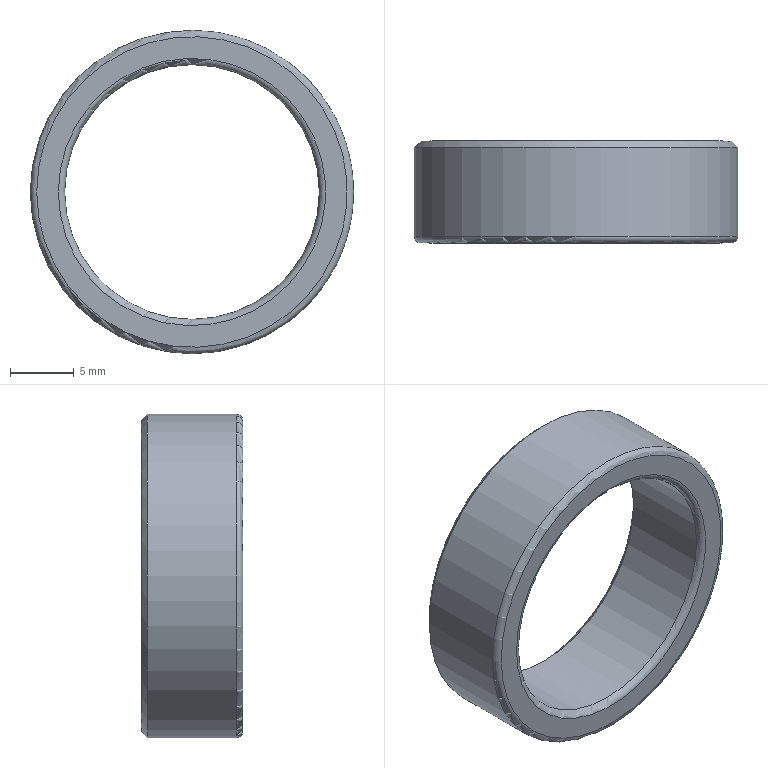Part | STEP file | BK-20_id1246_x_t | 1 solid | 8 faces | box 25.4 x 8 x 25.4 mm | volume 1515 mm3 | cylinder 2 | cone 2 | torus 2 | plane 2 | commonest cylinder face diameters 20 x1 25.4 x1
STEP:
#1=CARTESIAN_POINT('',(0.,0.,0.));
#2=DIRECTION('',(0.,0.,1.));
#3=DIRECTION('',(1.,0.,0.));
#4=AXIS2_PLACEMENT_3D('',#1,#2,#3);
#5=CARTESIAN_POINT('',(-258.5,542.436,-165.5));
#6=VERTEX_POINT('',#5);
#7=CARTESIAN_POINT('',(-278.5,542.436,-165.5));
#8=VERTEX_POINT('',#7);
#9=CARTESIAN_POINT('',(-268.5,542.436,-165.5));
#10=DIRECTION('',(0.,1.,0.));
#11=DIRECTION('',(1.,0.,0.));
#12=AXIS2_PLACEMENT_3D('',#9,#10,#11);
#13=CIRCLE('',#12,10.);
#14=CARTESIAN_POINT('',(-268.5,526.874,-165.5));
#15=DIRECTION('',(0.,-1.,0.));
#16=DIRECTION('',(1.,0.,0.));
#17=AXIS2_PLACEMENT_3D('',#14,#15,#16);
#18=CYLINDRICAL_SURFACE('',#17,10.);
#19=CARTESIAN_POINT('',(6.283,-15.562));
#20=DIRECTION('',(-1.,0.));
#21=VECTOR('',#20,1.);
#22=LINE('',#19,#21);
#23=(GEOMETRIC_REPRESENTATION_CONTEXT(2)PARAMETRIC_REPRESENTATION_CONTEXT()REPRESENTATION_CONTEXT('',''));
#24=DEFINITIONAL_REPRESENTATION('',(#22),#23);
#25=PCURVE('',#18,#24);
#26=CARTESIAN_POINT('',(-268.5,542.436,-165.5));
#27=DIRECTION('',(0.,1.,0.));
#28=DIRECTION('',(-1.,0.,0.));
#29=AXIS2_PLACEMENT_3D('',#26,#27,#28);
#30=TOROIDAL_SURFACE('',#29,10.5,0.5);
#31=CARTESIAN_POINT('',(3.142,3.142));
#32=DIRECTION('',(1.,0.));
#33=VECTOR('',#32,1.);
#34=LINE('',#31,#33);
#35=(GEOMETRIC_REPRESENTATION_CONTEXT(2)PARAMETRIC_REPRESENTATION_CONTEXT()REPRESENTATION_CONTEXT('',''));
#36=DEFINITIONAL_REPRESENTATION('',(#34),#35);
#37=PCURVE('',#30,#36);
#38=SURFACE_CURVE('',#13,(#25,#37),.PCURVE_S1.);
#39=EDGE_CURVE('',#6,#8,#38,.T.);
#40=ORIENTED_EDGE('',*,*,#39,.T.);
#41=CARTESIAN_POINT('',(-268.5,542.436,-165.5));
#42=DIRECTION('',(0.,1.,0.));
#43=DIRECTION('',(1.,0.,0.));
#44=AXIS2_PLACEMENT_3D('',#41,#42,#43);
#45=CIRCLE('',#44,10.);
#46=CARTESIAN_POINT('',(6.283,-15.562));
#47=DIRECTION('',(-1.,0.));
#48=VECTOR('',#47,1.);
#49=LINE('',#46,#48);
#50=(GEOMETRIC_REPRESENTATION_CONTEXT(2)PARAMETRIC_REPRESENTATION_CONTEXT()REPRESENTATION_CONTEXT('',''));
#51=DEFINITIONAL_REPRESENTATION('',(#49),#50);
#52=PCURVE('',#18,#51);
#53=CARTESIAN_POINT('',(-3.142,3.142));
#54=DIRECTION('',(1.,0.));
#55=VECTOR('',#54,1.);
#56=LINE('',#53,#55);
#57=(GEOMETRIC_REPRESENTATION_CONTEXT(2)PARAMETRIC_REPRESENTATION_CONTEXT()REPRESENTATION_CONTEXT('',''));
#58=DEFINITIONAL_REPRESENTATION('',(#56),#57);
#59=PCURVE('',#30,#58);
#60=SURFACE_CURVE('',#45,(#52,#59),.PCURVE_S1.);
#61=EDGE_CURVE('',#8,#6,#60,.T.);
#62=ORIENTED_EDGE('',*,*,#61,.T.);
#63=CARTESIAN_POINT('',(-258.5,549.436,-165.5));
#64=VERTEX_POINT('',#63);
#65=CARTESIAN_POINT('',(-258.5,549.436,-165.5));
#66=CARTESIAN_POINT('',(-258.5,542.436,-165.5));
#67=B_SPLINE_CURVE_WITH_KNOTS('',1,(#65,#66),.UNSPECIFIED.,.F.,.F.,(2,2),(-22.562,-15.562),.PIECEWISE_BEZIER_KNOTS.);
#68=CARTESIAN_POINT('',(0.,0.));
#69=DIRECTION('',(0.,1.));
#70=VECTOR('',#69,1.);
#71=LINE('',#68,#70);
#72=(GEOMETRIC_REPRESENTATION_CONTEXT(2)PARAMETRIC_REPRESENTATION_CONTEXT()REPRESENTATION_CONTEXT('',''));
#73=DEFINITIONAL_REPRESENTATION('',(#71),#72);
#74=PCURVE('',#18,#73);
#75=CARTESIAN_POINT('',(6.283,0.));
#76=DIRECTION('',(0.,1.));
#77=VECTOR('',#76,1.);
#78=LINE('',#75,#77);
#79=(GEOMETRIC_REPRESENTATION_CONTEXT(2)PARAMETRIC_REPRESENTATION_CONTEXT()REPRESENTATION_CONTEXT('',''));
#80=DEFINITIONAL_REPRESENTATION('',(#78),#79);
#81=PCURVE('',#18,#80);
#82=SEAM_CURVE('',#67,(#74,#81),.PCURVE_S1.);
#83=EDGE_CURVE('',#64,#6,#82,.T.);
#84=ORIENTED_EDGE('',*,*,#83,.F.);
#85=CARTESIAN_POINT('',(-278.5,549.436,-165.5));
#86=VERTEX_POINT('',#85);
#87=CARTESIAN_POINT('',(-268.5,549.436,-165.5));
#88=DIRECTION('',(0.,1.,0.));
#89=DIRECTION('',(-1.,0.,0.));
#90=AXIS2_PLACEMENT_3D('',#87,#88,#89);
#91=CIRCLE('',#90,10.);
#92=CARTESIAN_POINT('',(3.142,-22.562));
#93=DIRECTION('',(-1.,0.));
#94=VECTOR('',#93,1.);
#95=LINE('',#92,#94);
#96=(GEOMETRIC_REPRESENTATION_CONTEXT(2)PARAMETRIC_REPRESENTATION_CONTEXT()REPRESENTATION_CONTEXT('',''));
#97=DEFINITIONAL_REPRESENTATION('',(#95),#96);
#98=PCURVE('',#18,#97);
#99=CARTESIAN_POINT('',(-268.5,549.936,-165.5));
#100=DIRECTION('',(0.,1.,0.));
#101=DIRECTION('',(-1.,0.,0.));
#102=AXIS2_PLACEMENT_3D('',#99,#100,#101);
#103=CONICAL_SURFACE('',#102,10.5,0.7854);
#104=CARTESIAN_POINT('',(0.,-0.5));
#105=DIRECTION('',(1.,0.));
#106=VECTOR('',#105,1.);
#107=LINE('',#104,#106);
#108=(GEOMETRIC_REPRESENTATION_CONTEXT(2)PARAMETRIC_REPRESENTATION_CONTEXT()REPRESENTATION_CONTEXT('',''));
#109=DEFINITIONAL_REPRESENTATION('',(#107),#108);
#110=PCURVE('',#103,#109);
#111=SURFACE_CURVE('',#91,(#98,#110),.PCURVE_S1.);
#112=EDGE_CURVE('',#86,#64,#111,.T.);
#113=ORIENTED_EDGE('',*,*,#112,.F.);
#114=CARTESIAN_POINT('',(-268.5,549.436,-165.5));
#115=DIRECTION('',(0.,1.,0.));
#116=DIRECTION('',(-1.,0.,0.));
#117=AXIS2_PLACEMENT_3D('',#114,#115,#116);
#118=CIRCLE('',#117,10.);
#119=CARTESIAN_POINT('',(9.425,-22.562));
#120=DIRECTION('',(-1.,0.));
#121=VECTOR('',#120,1.);
#122=LINE('',#119,#121);
#123=(GEOMETRIC_REPRESENTATION_CONTEXT(2)PARAMETRIC_REPRESENTATION_CONTEXT()REPRESENTATION_CONTEXT('',''));
#124=DEFINITIONAL_REPRESENTATION('',(#122),#123);
#125=PCURVE('',#18,#124);
#126=CARTESIAN_POINT('',(0.,-0.5));
#127=DIRECTION('',(1.,0.));
#128=VECTOR('',#127,1.);
#129=LINE('',#126,#128);
#130=(GEOMETRIC_REPRESENTATION_CONTEXT(2)PARAMETRIC_REPRESENTATION_CONTEXT()REPRESENTATION_CONTEXT('',''));
#131=DEFINITIONAL_REPRESENTATION('',(#129),#130);
#132=PCURVE('',#103,#131);
#133=SURFACE_CURVE('',#118,(#125,#132),.PCURVE_S1.);
#134=EDGE_CURVE('',#64,#86,#133,.T.);
#135=ORIENTED_EDGE('',*,*,#134,.F.);
#136=ORIENTED_EDGE('',*,*,#83,.T.);
#137=EDGE_LOOP('',(#40,#62,#84,#113,#135,#136));
#138=FACE_BOUND('',#137,.F.);
#139=ADVANCED_FACE('',(#138),#18,.F.);
#140=ORIENTED_EDGE('',*,*,#134,.T.);
#141=CARTESIAN_POINT('',(-279.,549.936,-165.5));
#142=VERTEX_POINT('',#141);
#143=CARTESIAN_POINT('',(-278.5,549.436,-165.5));
#144=CARTESIAN_POINT('',(-279.,549.936,-165.5));
#145=B_SPLINE_CURVE_WITH_KNOTS('',1,(#143,#144),.UNSPECIFIED.,.F.,.F.,(2,2),(-0.7071,0.),.PIECEWISE_BEZIER_KNOTS.);
#146=CARTESIAN_POINT('',(6.283,0.));
#147=DIRECTION('',(0.,1.));
#148=VECTOR('',#147,1.);
#149=LINE('',#146,#148);
#150=(GEOMETRIC_REPRESENTATION_CONTEXT(2)PARAMETRIC_REPRESENTATION_CONTEXT()REPRESENTATION_CONTEXT('',''));
#151=DEFINITIONAL_REPRESENTATION('',(#149),#150);
#152=PCURVE('',#103,#151);
#153=CARTESIAN_POINT('',(0.,0.));
#154=DIRECTION('',(0.,1.));
#155=VECTOR('',#154,1.);
#156=LINE('',#153,#155);
#157=(GEOMETRIC_REPRESENTATION_CONTEXT(2)PARAMETRIC_REPRESENTATION_CONTEXT()REPRESENTATION_CONTEXT('',''));
#158=DEFINITIONAL_REPRESENTATION('',(#156),#157);
#159=PCURVE('',#103,#158);
#160=SEAM_CURVE('',#145,(#152,#159),.PCURVE_S1.);
#161=EDGE_CURVE('',#86,#142,#160,.T.);
#162=ORIENTED_EDGE('',*,*,#161,.T.);
#163=CARTESIAN_POINT('',(-268.5,549.936,-165.5));
#164=DIRECTION('',(0.,1.,0.));
#165=DIRECTION('',(-1.,0.,0.));
#166=AXIS2_PLACEMENT_3D('',#163,#164,#165);
#167=CIRCLE('',#166,10.5);
#168=CARTESIAN_POINT('',(0.,0.));
#169=DIRECTION('',(1.,0.));
#170=VECTOR('',#169,1.);
#171=LINE('',#168,#170);
#172=(GEOMETRIC_REPRESENTATION_CONTEXT(2)PARAMETRIC_REPRESENTATION_CONTEXT()REPRESENTATION_CONTEXT('',''));
#173=DEFINITIONAL_REPRESENTATION('',(#171),#172);
#174=PCURVE('',#103,#173);
#175=CARTESIAN_POINT('',(-268.5,549.936,-152.8));
#176=DIRECTION('',(0.,-1.,0.));
#177=DIRECTION('',(1.,0.,0.));
#178=AXIS2_PLACEMENT_3D('',#175,#176,#177);
#179=PLANE('',#178);
#180=CARTESIAN_POINT('',(-10.5,-12.7));
#181=CARTESIAN_POINT('',(-10.5,5.487));
#182=CARTESIAN_POINT('',(5.25,-3.607));
#183=CARTESIAN_POINT('',(21.,-12.7));
#184=CARTESIAN_POINT('',(5.25,-21.793));
#185=CARTESIAN_POINT('',(-10.5,-30.887));
#186=CARTESIAN_POINT('',(-10.5,-12.7));
#187=(BOUNDED_CURVE()B_SPLINE_CURVE(2,(#180,#181,#182,#183,#184,#185,#186),.UNSPECIFIED.,.T.,.F.)B_SPLINE_CURVE_WITH_KNOTS((1,2,2,2,2,1),(-2.094,0.,2.094,4.189,6.283,8.378),.UNSPECIFIED.)CURVE()GEOMETRIC_REPRESENTATION_ITEM()RATIONAL_B_SPLINE_CURVE((1.,0.5,1.,0.5,1.,0.5,1.))REPRESENTATION_ITEM(''));
#188=(GEOMETRIC_REPRESENTATION_CONTEXT(2)PARAMETRIC_REPRESENTATION_CONTEXT()REPRESENTATION_CONTEXT('',''));
#189=DEFINITIONAL_REPRESENTATION('',(#187),#188);
#190=PCURVE('',#179,#189);
#191=SURFACE_CURVE('',#167,(#174,#190),.PCURVE_S1.);
#192=EDGE_CURVE('',#142,#142,#191,.T.);
#193=ORIENTED_EDGE('',*,*,#192,.F.);
#194=ORIENTED_EDGE('',*,*,#161,.F.);
#195=ORIENTED_EDGE('',*,*,#112,.T.);
#196=EDGE_LOOP('',(#140,#162,#193,#194,#195));
#197=FACE_BOUND('',#196,.F.);
#198=ADVANCED_FACE('',(#197),#103,.F.);
#199=ORIENTED_EDGE('',*,*,#39,.T.);
#200=CARTESIAN_POINT('',(-279.,541.936,-165.5));
#201=VERTEX_POINT('',#200);
#202=CARTESIAN_POINT('',(-278.5,542.436,-165.5));
#203=CARTESIAN_POINT('',(-278.5,542.302,-165.5));
#204=CARTESIAN_POINT('',(-278.543,542.172,-165.5));
#205=CARTESIAN_POINT('',(-278.624,542.06,-165.5));
#206=CARTESIAN_POINT('',(-278.736,541.978,-165.5));
#207=CARTESIAN_POINT('',(-278.866,541.936,-165.5));
#208=CARTESIAN_POINT('',(-279.,541.936,-165.5));
#209=(BOUNDED_CURVE()B_SPLINE_CURVE(6,(#202,#203,#204,#205,#206,#207,#208),.UNSPECIFIED.,.F.,.F.)B_SPLINE_CURVE_WITH_KNOTS((7,7),(3.142,4.712),.PIECEWISE_BEZIER_KNOTS.)CURVE()GEOMETRIC_REPRESENTATION_ITEM()RATIONAL_B_SPLINE_CURVE((1.031,1.01,0.9979,0.994,0.9979,1.01,1.031))REPRESENTATION_ITEM(''));
#210=CARTESIAN_POINT('',(6.283,0.));
#211=DIRECTION('',(0.,1.));
#212=VECTOR('',#211,1.);
#213=LINE('',#210,#212);
#214=(GEOMETRIC_REPRESENTATION_CONTEXT(2)PARAMETRIC_REPRESENTATION_CONTEXT()REPRESENTATION_CONTEXT('',''));
#215=DEFINITIONAL_REPRESENTATION('',(#213),#214);
#216=PCURVE('',#30,#215);
#217=CARTESIAN_POINT('',(0.,0.));
#218=DIRECTION('',(0.,1.));
#219=VECTOR('',#218,1.);
#220=LINE('',#217,#219);
#221=(GEOMETRIC_REPRESENTATION_CONTEXT(2)PARAMETRIC_REPRESENTATION_CONTEXT()REPRESENTATION_CONTEXT('',''));
#222=DEFINITIONAL_REPRESENTATION('',(#220),#221);
#223=PCURVE('',#30,#222);
#224=SEAM_CURVE('',#209,(#216,#223),.PCURVE_S1.);
#225=EDGE_CURVE('',#8,#201,#224,.T.);
#226=ORIENTED_EDGE('',*,*,#225,.T.);
#227=CARTESIAN_POINT('',(-268.5,541.936,-165.5));
#228=DIRECTION('',(0.,-1.,0.));
#229=DIRECTION('',(-1.,0.,0.));
#230=AXIS2_PLACEMENT_3D('',#227,#228,#229);
#231=CIRCLE('',#230,10.5);
#232=CARTESIAN_POINT('',(6.283,4.712));
#233=DIRECTION('',(-1.,0.));
#234=VECTOR('',#233,1.);
#235=LINE('',#232,#234);
#236=(GEOMETRIC_REPRESENTATION_CONTEXT(2)PARAMETRIC_REPRESENTATION_CONTEXT()REPRESENTATION_CONTEXT('',''));
#237=DEFINITIONAL_REPRESENTATION('',(#235),#236);
#238=PCURVE('',#30,#237);
#239=CARTESIAN_POINT('',(-268.5,541.936,-152.8));
#240=DIRECTION('',(0.,1.,0.));
#241=DIRECTION('',(-1.,0.,0.));
#242=AXIS2_PLACEMENT_3D('',#239,#240,#241);
#243=PLANE('',#242);
#244=CARTESIAN_POINT('',(10.5,-12.7));
#245=CARTESIAN_POINT('',(10.5,-30.887));
#246=CARTESIAN_POINT('',(-5.25,-21.793));
#247=CARTESIAN_POINT('',(-21.,-12.7));
#248=CARTESIAN_POINT('',(-5.25,-3.607));
#249=CARTESIAN_POINT('',(10.5,5.487));
#250=CARTESIAN_POINT('',(10.5,-12.7));
#251=(BOUNDED_CURVE()B_SPLINE_CURVE(2,(#244,#245,#246,#247,#248,#249,#250),.UNSPECIFIED.,.T.,.F.)B_SPLINE_CURVE_WITH_KNOTS((1,2,2,2,2,1),(-2.094,0.,2.094,4.189,6.283,8.378),.UNSPECIFIED.)CURVE()GEOMETRIC_REPRESENTATION_ITEM()RATIONAL_B_SPLINE_CURVE((1.,0.5,1.,0.5,1.,0.5,1.))REPRESENTATION_ITEM(''));
#252=(GEOMETRIC_REPRESENTATION_CONTEXT(2)PARAMETRIC_REPRESENTATION_CONTEXT()REPRESENTATION_CONTEXT('',''));
#253=DEFINITIONAL_REPRESENTATION('',(#251),#252);
#254=PCURVE('',#243,#253);
#255=SURFACE_CURVE('',#231,(#238,#254),.PCURVE_S1.);
#256=EDGE_CURVE('',#201,#201,#255,.T.);
#257=ORIENTED_EDGE('',*,*,#256,.T.);
#258=ORIENTED_EDGE('',*,*,#225,.F.);
#259=ORIENTED_EDGE('',*,*,#61,.T.);
#260=EDGE_LOOP('',(#199,#226,#257,#258,#259));
#261=FACE_BOUND('',#260,.T.);
#262=ADVANCED_FACE('',(#261),#30,.T.);
#263=ORIENTED_EDGE('',*,*,#192,.F.);
#264=EDGE_LOOP('',(#263));
#265=FACE_BOUND('',#264,.T.);
#266=CARTESIAN_POINT('',(-256.3,549.936,-165.5));
#267=VERTEX_POINT('',#266);
#268=CARTESIAN_POINT('',(-268.5,549.936,-165.5));
#269=DIRECTION('',(0.,-1.,0.));
#270=DIRECTION('',(1.,0.,0.));
#271=AXIS2_PLACEMENT_3D('',#268,#269,#270);
#272=CIRCLE('',#271,12.2);
#273=CARTESIAN_POINT('',(0.,-12.7));
#274=DIRECTION('',(1.,0.));
#275=AXIS2_PLACEMENT_2D('',#273,#274);
#276=CIRCLE('',#275,12.2);
#277=(GEOMETRIC_REPRESENTATION_CONTEXT(2)PARAMETRIC_REPRESENTATION_CONTEXT()REPRESENTATION_CONTEXT('',''));
#278=DEFINITIONAL_REPRESENTATION('',(#276),#277);
#279=PCURVE('',#179,#278);
#280=CARTESIAN_POINT('',(-268.5,549.436,-165.5));
#281=DIRECTION('',(0.,-1.,0.));
#282=DIRECTION('',(1.,0.,0.));
#283=AXIS2_PLACEMENT_3D('',#280,#281,#282);
#284=CONICAL_SURFACE('',#283,12.7,0.7854);
#285=CARTESIAN_POINT('',(0.,-0.5));
#286=DIRECTION('',(1.,0.));
#287=VECTOR('',#286,1.);
#288=LINE('',#285,#287);
#289=(GEOMETRIC_REPRESENTATION_CONTEXT(2)PARAMETRIC_REPRESENTATION_CONTEXT()REPRESENTATION_CONTEXT('',''));
#290=DEFINITIONAL_REPRESENTATION('',(#288),#289);
#291=PCURVE('',#284,#290);
#292=SURFACE_CURVE('',#272,(#279,#291),.PCURVE_S1.);
#293=EDGE_CURVE('',#267,#267,#292,.T.);
#294=ORIENTED_EDGE('',*,*,#293,.F.);
#295=EDGE_LOOP('',(#294));
#296=FACE_BOUND('',#295,.T.);
#297=ADVANCED_FACE('',(#265,#296),#179,.F.);
#298=ORIENTED_EDGE('',*,*,#256,.F.);
#299=EDGE_LOOP('',(#298));
#300=FACE_BOUND('',#299,.T.);
#301=CARTESIAN_POINT('',(-280.7,541.936,-165.5));
#302=VERTEX_POINT('',#301);
#303=CARTESIAN_POINT('',(-268.5,541.936,-165.5));
#304=DIRECTION('',(0.,1.,0.));
#305=DIRECTION('',(-1.,0.,0.));
#306=AXIS2_PLACEMENT_3D('',#303,#304,#305);
#307=CIRCLE('',#306,12.2);
#308=CARTESIAN_POINT('',(0.,-12.7));
#309=DIRECTION('',(1.,0.));
#310=AXIS2_PLACEMENT_2D('',#308,#309);
#311=CIRCLE('',#310,12.2);
#312=(GEOMETRIC_REPRESENTATION_CONTEXT(2)PARAMETRIC_REPRESENTATION_CONTEXT()REPRESENTATION_CONTEXT('',''));
#313=DEFINITIONAL_REPRESENTATION('',(#311),#312);
#314=PCURVE('',#243,#313);
#315=CARTESIAN_POINT('',(-268.5,542.436,-165.5));
#316=DIRECTION('',(0.,1.,0.));
#317=DIRECTION('',(-1.,0.,0.));
#318=AXIS2_PLACEMENT_3D('',#315,#316,#317);
#319=TOROIDAL_SURFACE('',#318,12.2,0.5);
#320=CARTESIAN_POINT('',(0.,4.712));
#321=DIRECTION('',(1.,0.));
#322=VECTOR('',#321,1.);
#323=LINE('',#320,#322);
#324=(GEOMETRIC_REPRESENTATION_CONTEXT(2)PARAMETRIC_REPRESENTATION_CONTEXT()REPRESENTATION_CONTEXT('',''));
#325=DEFINITIONAL_REPRESENTATION('',(#323),#324);
#326=PCURVE('',#319,#325);
#327=SURFACE_CURVE('',#307,(#314,#326),.PCURVE_S1.);
#328=EDGE_CURVE('',#302,#302,#327,.T.);
#329=ORIENTED_EDGE('',*,*,#328,.F.);
#330=EDGE_LOOP('',(#329));
#331=FACE_BOUND('',#330,.T.);
#332=ADVANCED_FACE('',(#300,#331),#243,.F.);
#333=ORIENTED_EDGE('',*,*,#293,.T.);
#334=CARTESIAN_POINT('',(-255.8,549.436,-165.5));
#335=VERTEX_POINT('',#334);
#336=CARTESIAN_POINT('',(-256.3,549.936,-165.5));
#337=CARTESIAN_POINT('',(-255.8,549.436,-165.5));
#338=B_SPLINE_CURVE_WITH_KNOTS('',1,(#336,#337),.UNSPECIFIED.,.F.,.F.,(2,2),(-0.7071,0.),.PIECEWISE_BEZIER_KNOTS.);
#339=CARTESIAN_POINT('',(6.283,0.));
#340=DIRECTION('',(0.,1.));
#341=VECTOR('',#340,1.);
#342=LINE('',#339,#341);
#343=(GEOMETRIC_REPRESENTATION_CONTEXT(2)PARAMETRIC_REPRESENTATION_CONTEXT()REPRESENTATION_CONTEXT('',''));
#344=DEFINITIONAL_REPRESENTATION('',(#342),#343);
#345=PCURVE('',#284,#344);
#346=CARTESIAN_POINT('',(0.,0.));
#347=DIRECTION('',(0.,1.));
#348=VECTOR('',#347,1.);
#349=LINE('',#346,#348);
#350=(GEOMETRIC_REPRESENTATION_CONTEXT(2)PARAMETRIC_REPRESENTATION_CONTEXT()REPRESENTATION_CONTEXT('',''));
#351=DEFINITIONAL_REPRESENTATION('',(#349),#350);
#352=PCURVE('',#284,#351);
#353=SEAM_CURVE('',#338,(#345,#352),.PCURVE_S1.);
#354=EDGE_CURVE('',#267,#335,#353,.T.);
#355=ORIENTED_EDGE('',*,*,#354,.T.);
#356=CARTESIAN_POINT('',(-268.5,549.436,-165.5));
#357=DIRECTION('',(0.,-1.,0.));
#358=DIRECTION('',(1.,0.,0.));
#359=AXIS2_PLACEMENT_3D('',#356,#357,#358);
#360=CIRCLE('',#359,12.7);
#361=CARTESIAN_POINT('',(0.,0.));
#362=DIRECTION('',(1.,0.));
#363=VECTOR('',#362,1.);
#364=LINE('',#361,#363);
#365=(GEOMETRIC_REPRESENTATION_CONTEXT(2)PARAMETRIC_REPRESENTATION_CONTEXT()REPRESENTATION_CONTEXT('',''));
#366=DEFINITIONAL_REPRESENTATION('',(#364),#365);
#367=PCURVE('',#284,#366);
#368=CARTESIAN_POINT('',(-268.5,526.874,-165.5));
#369=DIRECTION('',(0.,-1.,0.));
#370=DIRECTION('',(1.,0.,0.));
#371=AXIS2_PLACEMENT_3D('',#368,#369,#370);
#372=CYLINDRICAL_SURFACE('',#371,12.7);
#373=CARTESIAN_POINT('',(0.,-22.562));
#374=DIRECTION('',(1.,0.));
#375=VECTOR('',#374,1.);
#376=LINE('',#373,#375);
#377=(GEOMETRIC_REPRESENTATION_CONTEXT(2)PARAMETRIC_REPRESENTATION_CONTEXT()REPRESENTATION_CONTEXT('',''));
#378=DEFINITIONAL_REPRESENTATION('',(#376),#377);
#379=PCURVE('',#372,#378);
#380=SURFACE_CURVE('',#360,(#367,#379),.PCURVE_S1.);
#381=EDGE_CURVE('',#335,#335,#380,.T.);
#382=ORIENTED_EDGE('',*,*,#381,.F.);
#383=ORIENTED_EDGE('',*,*,#354,.F.);
#384=EDGE_LOOP('',(#333,#355,#382,#383));
#385=FACE_BOUND('',#384,.T.);
#386=ADVANCED_FACE('',(#385),#284,.T.);
#387=CARTESIAN_POINT('',(-281.2,542.436,-165.5));
#388=VERTEX_POINT('',#387);
#389=CARTESIAN_POINT('',(-255.8,542.436,-165.5));
#390=VERTEX_POINT('',#389);
#391=CARTESIAN_POINT('',(-268.5,542.436,-165.5));
#392=DIRECTION('',(0.,1.,0.));
#393=DIRECTION('',(1.,0.,0.));
#394=AXIS2_PLACEMENT_3D('',#391,#392,#393);
#395=CIRCLE('',#394,12.7);
#396=CARTESIAN_POINT('',(-3.142,6.283));
#397=DIRECTION('',(1.,0.));
#398=VECTOR('',#397,1.);
#399=LINE('',#396,#398);
#400=(GEOMETRIC_REPRESENTATION_CONTEXT(2)PARAMETRIC_REPRESENTATION_CONTEXT()REPRESENTATION_CONTEXT('',''));
#401=DEFINITIONAL_REPRESENTATION('',(#399),#400);
#402=PCURVE('',#319,#401);
#403=CARTESIAN_POINT('',(6.283,-15.562));
#404=DIRECTION('',(-1.,0.));
#405=VECTOR('',#404,1.);
#406=LINE('',#403,#405);
#407=(GEOMETRIC_REPRESENTATION_CONTEXT(2)PARAMETRIC_REPRESENTATION_CONTEXT()REPRESENTATION_CONTEXT('',''));
#408=DEFINITIONAL_REPRESENTATION('',(#406),#407);
#409=PCURVE('',#372,#408);
#410=SURFACE_CURVE('',#395,(#402,#409),.PCURVE_S1.);
#411=EDGE_CURVE('',#388,#390,#410,.T.);
#412=ORIENTED_EDGE('',*,*,#411,.F.);
#413=CARTESIAN_POINT('',(-280.7,541.936,-165.5));
#414=CARTESIAN_POINT('',(-280.834,541.936,-165.5));
#415=CARTESIAN_POINT('',(-280.964,541.978,-165.5));
#416=CARTESIAN_POINT('',(-281.076,542.06,-165.5));
#417=CARTESIAN_POINT('',(-281.157,542.172,-165.5));
#418=CARTESIAN_POINT('',(-281.2,542.302,-165.5));
#419=CARTESIAN_POINT('',(-281.2,542.436,-165.5));
#420=(BOUNDED_CURVE()B_SPLINE_CURVE(6,(#413,#414,#415,#416,#417,#418,#419),.UNSPECIFIED.,.F.,.F.)B_SPLINE_CURVE_WITH_KNOTS((7,7),(-1.571,0.),.PIECEWISE_BEZIER_KNOTS.)CURVE()GEOMETRIC_REPRESENTATION_ITEM()RATIONAL_B_SPLINE_CURVE((1.031,1.01,0.9979,0.994,0.9979,1.01,1.031))REPRESENTATION_ITEM(''));
#421=CARTESIAN_POINT('',(0.,6.283));
#422=DIRECTION('',(0.,1.));
#423=VECTOR('',#422,1.);
#424=LINE('',#421,#423);
#425=(GEOMETRIC_REPRESENTATION_CONTEXT(2)PARAMETRIC_REPRESENTATION_CONTEXT()REPRESENTATION_CONTEXT('',''));
#426=DEFINITIONAL_REPRESENTATION('',(#424),#425);
#427=PCURVE('',#319,#426);
#428=CARTESIAN_POINT('',(6.283,6.283));
#429=DIRECTION('',(0.,1.));
#430=VECTOR('',#429,1.);
#431=LINE('',#428,#430);
#432=(GEOMETRIC_REPRESENTATION_CONTEXT(2)PARAMETRIC_REPRESENTATION_CONTEXT()REPRESENTATION_CONTEXT('',''));
#433=DEFINITIONAL_REPRESENTATION('',(#431),#432);
#434=PCURVE('',#319,#433);
#435=SEAM_CURVE('',#420,(#427,#434),.PCURVE_S1.);
#436=EDGE_CURVE('',#302,#388,#435,.T.);
#437=ORIENTED_EDGE('',*,*,#436,.F.);
#438=ORIENTED_EDGE('',*,*,#328,.T.);
#439=ORIENTED_EDGE('',*,*,#436,.T.);
#440=CARTESIAN_POINT('',(-268.5,542.436,-165.5));
#441=DIRECTION('',(0.,1.,0.));
#442=DIRECTION('',(1.,0.,0.));
#443=AXIS2_PLACEMENT_3D('',#440,#441,#442);
#444=CIRCLE('',#443,12.7);
#445=CARTESIAN_POINT('',(3.142,6.283));
#446=DIRECTION('',(1.,0.));
#447=VECTOR('',#446,1.);
#448=LINE('',#445,#447);
#449=(GEOMETRIC_REPRESENTATION_CONTEXT(2)PARAMETRIC_REPRESENTATION_CONTEXT()REPRESENTATION_CONTEXT('',''));
#450=DEFINITIONAL_REPRESENTATION('',(#448),#449);
#451=PCURVE('',#319,#450);
#452=CARTESIAN_POINT('',(6.283,-15.562));
#453=DIRECTION('',(-1.,0.));
#454=VECTOR('',#453,1.);
#455=LINE('',#452,#454);
#456=(GEOMETRIC_REPRESENTATION_CONTEXT(2)PARAMETRIC_REPRESENTATION_CONTEXT()REPRESENTATION_CONTEXT('',''));
#457=DEFINITIONAL_REPRESENTATION('',(#455),#456);
#458=PCURVE('',#372,#457);
#459=SURFACE_CURVE('',#444,(#451,#458),.PCURVE_S1.);
#460=EDGE_CURVE('',#390,#388,#459,.T.);
#461=ORIENTED_EDGE('',*,*,#460,.F.);
#462=EDGE_LOOP('',(#412,#437,#438,#439,#461));
#463=FACE_BOUND('',#462,.T.);
#464=ADVANCED_FACE('',(#463),#319,.T.);
#465=ORIENTED_EDGE('',*,*,#381,.T.);
#466=CARTESIAN_POINT('',(-255.8,549.436,-165.5));
#467=CARTESIAN_POINT('',(-255.8,542.436,-165.5));
#468=B_SPLINE_CURVE_WITH_KNOTS('',1,(#466,#467),.UNSPECIFIED.,.F.,.F.,(2,2),(-22.562,-15.562),.PIECEWISE_BEZIER_KNOTS.);
#469=CARTESIAN_POINT('',(6.283,0.));
#470=DIRECTION('',(0.,1.));
#471=VECTOR('',#470,1.);
#472=LINE('',#469,#471);
#473=(GEOMETRIC_REPRESENTATION_CONTEXT(2)PARAMETRIC_REPRESENTATION_CONTEXT()REPRESENTATION_CONTEXT('',''));
#474=DEFINITIONAL_REPRESENTATION('',(#472),#473);
#475=PCURVE('',#372,#474);
#476=CARTESIAN_POINT('',(0.,0.));
#477=DIRECTION('',(0.,1.));
#478=VECTOR('',#477,1.);
#479=LINE('',#476,#478);
#480=(GEOMETRIC_REPRESENTATION_CONTEXT(2)PARAMETRIC_REPRESENTATION_CONTEXT()REPRESENTATION_CONTEXT('',''));
#481=DEFINITIONAL_REPRESENTATION('',(#479),#480);
#482=PCURVE('',#372,#481);
#483=SEAM_CURVE('',#468,(#475,#482),.PCURVE_S1.);
#484=EDGE_CURVE('',#335,#390,#483,.T.);
#485=ORIENTED_EDGE('',*,*,#484,.T.);
#486=ORIENTED_EDGE('',*,*,#460,.T.);
#487=ORIENTED_EDGE('',*,*,#411,.T.);
#488=ORIENTED_EDGE('',*,*,#484,.F.);
#489=EDGE_LOOP('',(#465,#485,#486,#487,#488));
#490=FACE_BOUND('',#489,.T.);
#491=ADVANCED_FACE('',(#490),#372,.T.);
#492=CLOSED_SHELL('',(#139,#198,#262,#297,#332,#386,#464,#491));
#493=MANIFOLD_SOLID_BREP('',#492);
#494=(LENGTH_UNIT()NAMED_UNIT(*)SI_UNIT(.MILLI.,.METRE.));
#495=UNCERTAINTY_MEASURE_WITH_UNIT(LENGTH_MEASURE(0.00001),#494,'','');
#496=(NAMED_UNIT(*)PLANE_ANGLE_UNIT()SI_UNIT($,.RADIAN.));
#497=(NAMED_UNIT(*)SI_UNIT($,.STERADIAN.)SOLID_ANGLE_UNIT());
#498=(GEOMETRIC_REPRESENTATION_CONTEXT(3)GLOBAL_UNCERTAINTY_ASSIGNED_CONTEXT((#495))GLOBAL_UNIT_ASSIGNED_CONTEXT((#494,#496,#497))REPRESENTATION_CONTEXT('',''));
#499=ADVANCED_BREP_SHAPE_REPRESENTATION('',(#4,#493),#498);